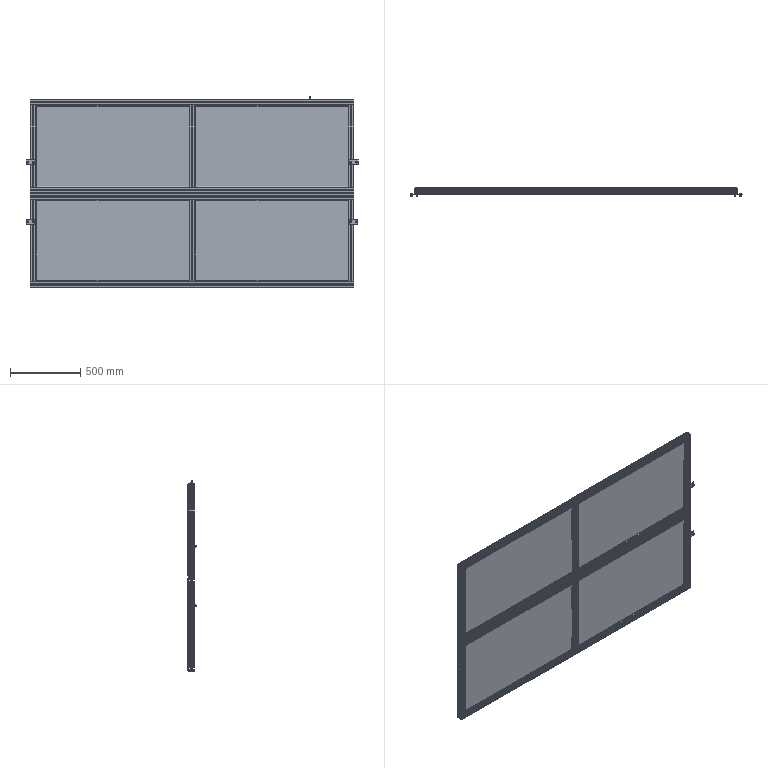Part | SolidWorks | features ReferencePattern 138, LocalLPattern 9, MirrorCompFeat 4 | 99 solids | 7791 faces | volume 23425150 mm3 | cylinder 4863 | plane 2784 | cone 144 | commonest cylinder face diameters 4 x3696 0.6 x264 6.6 x152 10 x136 6.8 x95 2 x88